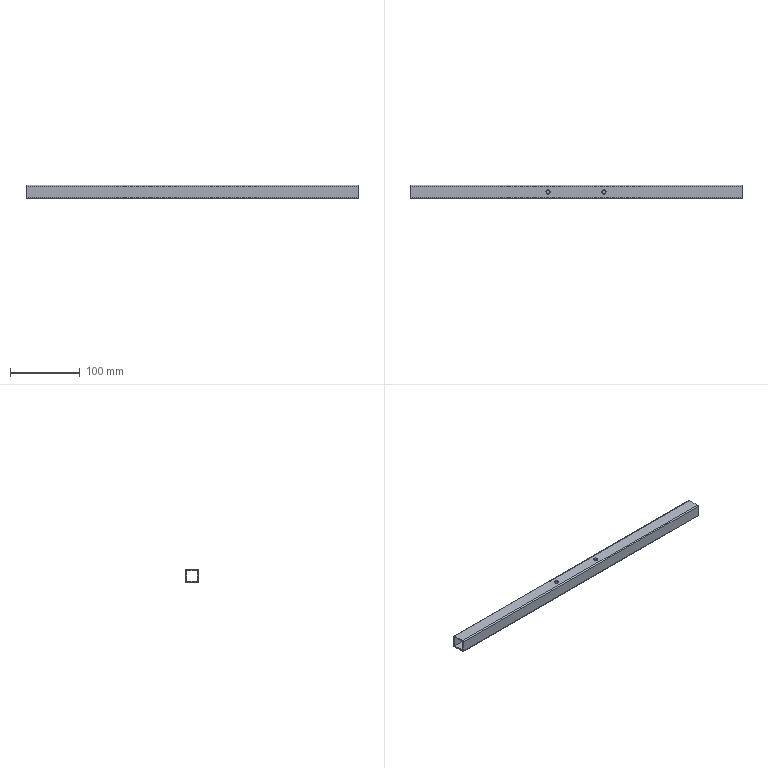Part | NX | features BREP 1 | 1 solid | 18 faces | box 474.98 x 19.05 x 19.05 mm | volume 63115 mm3 | plane 10 | cylinder 8 | commonest cylinder face diameters 3.175 x4 5.842 x4
STEP:
#1=CARTESIAN_POINT('',(-237.49,9.525,-7.938));
#2=VERTEX_POINT('',#1);
#3=CARTESIAN_POINT('',(-237.49,9.525,7.938));
#4=VERTEX_POINT('',#3);
#5=CARTESIAN_POINT('',(-237.49,9.525,-7.938));
#6=DIRECTION('',(0.,0.,1.));
#7=VECTOR('',#6,1000.);
#8=LINE('',#5,#7);
#9=EDGE_CURVE('',#2,#4,#8,.T.);
#10=ORIENTED_EDGE('',*,*,#9,.F.);
#11=CARTESIAN_POINT('',(-237.49,7.938,-9.525));
#12=VERTEX_POINT('',#11);
#13=CARTESIAN_POINT('',(-237.49,7.938,-7.938));
#14=DIRECTION('',(-1.,0.,0.));
#15=DIRECTION('',(0.,1.,0.));
#16=AXIS2_PLACEMENT_3D('',#13,#14,#15);
#17=CIRCLE('',#16,1.587);
#18=EDGE_CURVE('',#2,#12,#17,.T.);
#19=ORIENTED_EDGE('',*,*,#18,.T.);
#20=CARTESIAN_POINT('',(-237.49,-7.938,-9.525));
#21=VERTEX_POINT('',#20);
#22=CARTESIAN_POINT('',(-237.49,-7.938,-9.525));
#23=DIRECTION('',(0.,1.,0.));
#24=VECTOR('',#23,1000.);
#25=LINE('',#22,#24);
#26=EDGE_CURVE('',#21,#12,#25,.T.);
#27=ORIENTED_EDGE('',*,*,#26,.F.);
#28=CARTESIAN_POINT('',(-237.49,-9.525,-7.938));
#29=VERTEX_POINT('',#28);
#30=CARTESIAN_POINT('',(-237.49,-7.938,-7.938));
#31=DIRECTION('',(-1.,0.,0.));
#32=DIRECTION('',(0.,0.,-1.));
#33=AXIS2_PLACEMENT_3D('',#30,#31,#32);
#34=CIRCLE('',#33,1.587);
#35=EDGE_CURVE('',#21,#29,#34,.T.);
#36=ORIENTED_EDGE('',*,*,#35,.T.);
#37=CARTESIAN_POINT('',(-237.49,-9.525,7.938));
#38=VERTEX_POINT('',#37);
#39=CARTESIAN_POINT('',(-237.49,-9.525,7.938));
#40=DIRECTION('',(0.,0.,-1.));
#41=VECTOR('',#40,1000.);
#42=LINE('',#39,#41);
#43=EDGE_CURVE('',#38,#29,#42,.T.);
#44=ORIENTED_EDGE('',*,*,#43,.F.);
#45=CARTESIAN_POINT('',(-237.49,-7.938,9.525));
#46=VERTEX_POINT('',#45);
#47=CARTESIAN_POINT('',(-237.49,-7.938,7.938));
#48=DIRECTION('',(-1.,0.,0.));
#49=DIRECTION('',(0.,-1.,0.));
#50=AXIS2_PLACEMENT_3D('',#47,#48,#49);
#51=CIRCLE('',#50,1.587);
#52=EDGE_CURVE('',#38,#46,#51,.T.);
#53=ORIENTED_EDGE('',*,*,#52,.T.);
#54=CARTESIAN_POINT('',(-237.49,7.938,9.525));
#55=VERTEX_POINT('',#54);
#56=CARTESIAN_POINT('',(-237.49,7.938,9.525));
#57=DIRECTION('',(0.,-1.,0.));
#58=VECTOR('',#57,1000.);
#59=LINE('',#56,#58);
#60=EDGE_CURVE('',#55,#46,#59,.T.);
#61=ORIENTED_EDGE('',*,*,#60,.F.);
#62=CARTESIAN_POINT('',(-237.49,7.938,7.938));
#63=DIRECTION('',(-1.,0.,0.));
#64=DIRECTION('',(0.,0.,1.));
#65=AXIS2_PLACEMENT_3D('',#62,#63,#64);
#66=CIRCLE('',#65,1.587);
#67=EDGE_CURVE('',#55,#4,#66,.T.);
#68=ORIENTED_EDGE('',*,*,#67,.T.);
#69=EDGE_LOOP('',(#10,#19,#27,#36,#44,#53,#61,#68));
#70=FACE_BOUND('',#69,.T.);
#71=CARTESIAN_POINT('',(-237.49,7.544,7.544));
#72=VERTEX_POINT('',#71);
#73=CARTESIAN_POINT('',(-237.49,7.544,-7.544));
#74=VERTEX_POINT('',#73);
#75=CARTESIAN_POINT('',(-237.49,7.544,7.544));
#76=DIRECTION('',(0.,0.,-1.));
#77=VECTOR('',#76,1000.);
#78=LINE('',#75,#77);
#79=EDGE_CURVE('',#72,#74,#78,.T.);
#80=ORIENTED_EDGE('',*,*,#79,.F.);
#81=CARTESIAN_POINT('',(-237.49,-7.544,7.544));
#82=VERTEX_POINT('',#81);
#83=CARTESIAN_POINT('',(-237.49,-7.544,7.544));
#84=DIRECTION('',(0.,1.,0.));
#85=VECTOR('',#84,1000.);
#86=LINE('',#83,#85);
#87=EDGE_CURVE('',#82,#72,#86,.T.);
#88=ORIENTED_EDGE('',*,*,#87,.F.);
#89=CARTESIAN_POINT('',(-237.49,-7.544,-7.544));
#90=VERTEX_POINT('',#89);
#91=CARTESIAN_POINT('',(-237.49,-7.544,-7.544));
#92=DIRECTION('',(0.,0.,1.));
#93=VECTOR('',#92,1000.);
#94=LINE('',#91,#93);
#95=EDGE_CURVE('',#90,#82,#94,.T.);
#96=ORIENTED_EDGE('',*,*,#95,.F.);
#97=CARTESIAN_POINT('',(-237.49,7.544,-7.544));
#98=DIRECTION('',(0.,-1.,0.));
#99=VECTOR('',#98,1000.);
#100=LINE('',#97,#99);
#101=EDGE_CURVE('',#74,#90,#100,.T.);
#102=ORIENTED_EDGE('',*,*,#101,.F.);
#103=EDGE_LOOP('',(#80,#88,#96,#102));
#104=FACE_BOUND('',#103,.T.);
#105=CARTESIAN_POINT('',(-237.49,0.,0.));
#106=DIRECTION('',(1.,0.,0.));
#107=DIRECTION('',(0.,1.,0.));
#108=AXIS2_PLACEMENT_3D('',#105,#106,#107);
#109=PLANE('',#108);
#110=ADVANCED_FACE('',(#70,#104),#109,.F.);
#111=CARTESIAN_POINT('',(237.49,-7.544,-7.544));
#112=VERTEX_POINT('',#111);
#113=CARTESIAN_POINT('',(-237.49,-7.544,-7.544));
#114=DIRECTION('',(1.,0.,0.));
#115=VECTOR('',#114,1000.);
#116=LINE('',#113,#115);
#117=EDGE_CURVE('',#90,#112,#116,.T.);
#118=ORIENTED_EDGE('',*,*,#117,.T.);
#119=CARTESIAN_POINT('',(237.49,7.544,-7.544));
#120=VERTEX_POINT('',#119);
#121=CARTESIAN_POINT('',(237.49,7.544,-7.544));
#122=DIRECTION('',(0.,-1.,0.));
#123=VECTOR('',#122,1000.);
#124=LINE('',#121,#123);
#125=EDGE_CURVE('',#120,#112,#124,.T.);
#126=ORIENTED_EDGE('',*,*,#125,.F.);
#127=CARTESIAN_POINT('',(-237.49,7.544,-7.544));
#128=DIRECTION('',(1.,0.,0.));
#129=VECTOR('',#128,1000.);
#130=LINE('',#127,#129);
#131=EDGE_CURVE('',#74,#120,#130,.T.);
#132=ORIENTED_EDGE('',*,*,#131,.F.);
#133=ORIENTED_EDGE('',*,*,#101,.T.);
#134=EDGE_LOOP('',(#118,#126,#132,#133));
#135=FACE_BOUND('',#134,.T.);
#136=CARTESIAN_POINT('',(-237.49,7.544,-7.544));
#137=DIRECTION('',(0.,0.,1.));
#138=DIRECTION('',(1.,0.,0.));
#139=AXIS2_PLACEMENT_3D('',#136,#137,#138);
#140=PLANE('',#139);
#141=ADVANCED_FACE('',(#135),#140,.T.);
#142=ORIENTED_EDGE('',*,*,#131,.T.);
#143=CARTESIAN_POINT('',(237.49,7.544,7.544));
#144=VERTEX_POINT('',#143);
#145=CARTESIAN_POINT('',(237.49,7.544,7.544));
#146=DIRECTION('',(0.,0.,-1.));
#147=VECTOR('',#146,1000.);
#148=LINE('',#145,#147);
#149=EDGE_CURVE('',#144,#120,#148,.T.);
#150=ORIENTED_EDGE('',*,*,#149,.F.);
#151=CARTESIAN_POINT('',(-237.49,7.544,7.544));
#152=DIRECTION('',(1.,0.,0.));
#153=VECTOR('',#152,1000.);
#154=LINE('',#151,#153);
#155=EDGE_CURVE('',#72,#144,#154,.T.);
#156=ORIENTED_EDGE('',*,*,#155,.F.);
#157=ORIENTED_EDGE('',*,*,#79,.T.);
#158=EDGE_LOOP('',(#142,#150,#156,#157));
#159=FACE_BOUND('',#158,.T.);
#160=CARTESIAN_POINT('',(-237.49,7.544,7.544));
#161=DIRECTION('',(0.,-1.,0.));
#162=DIRECTION('',(0.,0.,-1.));
#163=AXIS2_PLACEMENT_3D('',#160,#161,#162);
#164=PLANE('',#163);
#165=ADVANCED_FACE('',(#159),#164,.T.);
#166=ORIENTED_EDGE('',*,*,#155,.T.);
#167=CARTESIAN_POINT('',(237.49,-7.544,7.544));
#168=VERTEX_POINT('',#167);
#169=CARTESIAN_POINT('',(237.49,-7.544,7.544));
#170=DIRECTION('',(0.,1.,0.));
#171=VECTOR('',#170,1000.);
#172=LINE('',#169,#171);
#173=EDGE_CURVE('',#168,#144,#172,.T.);
#174=ORIENTED_EDGE('',*,*,#173,.F.);
#175=CARTESIAN_POINT('',(-237.49,-7.544,7.544));
#176=DIRECTION('',(1.,0.,0.));
#177=VECTOR('',#176,1000.);
#178=LINE('',#175,#177);
#179=EDGE_CURVE('',#82,#168,#178,.T.);
#180=ORIENTED_EDGE('',*,*,#179,.F.);
#181=ORIENTED_EDGE('',*,*,#87,.T.);
#182=EDGE_LOOP('',(#166,#174,#180,#181));
#183=FACE_BOUND('',#182,.T.);
#184=CARTESIAN_POINT('',(-37.084,0.,7.544));
#185=VERTEX_POINT('',#184);
#186=CARTESIAN_POINT('',(-42.926,0.,7.544));
#187=VERTEX_POINT('',#186);
#188=CARTESIAN_POINT('',(-40.005,0.,7.544));
#189=DIRECTION('',(0.,0.,-1.));
#190=DIRECTION('',(1.,0.,0.));
#191=AXIS2_PLACEMENT_3D('',#188,#189,#190);
#192=CIRCLE('',#191,2.921);
#193=EDGE_CURVE('',#185,#187,#192,.T.);
#194=ORIENTED_EDGE('',*,*,#193,.F.);
#195=CARTESIAN_POINT('',(-40.005,0.,7.544));
#196=DIRECTION('',(0.,0.,-1.));
#197=DIRECTION('',(-1.,0.,0.));
#198=AXIS2_PLACEMENT_3D('',#195,#196,#197);
#199=CIRCLE('',#198,2.921);
#200=EDGE_CURVE('',#187,#185,#199,.T.);
#201=ORIENTED_EDGE('',*,*,#200,.F.);
#202=EDGE_LOOP('',(#194,#201));
#203=FACE_BOUND('',#202,.T.);
#204=CARTESIAN_POINT('',(42.926,0.,7.544));
#205=VERTEX_POINT('',#204);
#206=CARTESIAN_POINT('',(37.084,0.,7.544));
#207=VERTEX_POINT('',#206);
#208=CARTESIAN_POINT('',(40.005,0.,7.544));
#209=DIRECTION('',(0.,0.,-1.));
#210=DIRECTION('',(1.,0.,0.));
#211=AXIS2_PLACEMENT_3D('',#208,#209,#210);
#212=CIRCLE('',#211,2.921);
#213=EDGE_CURVE('',#205,#207,#212,.T.);
#214=ORIENTED_EDGE('',*,*,#213,.F.);
#215=CARTESIAN_POINT('',(40.005,0.,7.544));
#216=DIRECTION('',(0.,0.,-1.));
#217=DIRECTION('',(-1.,0.,0.));
#218=AXIS2_PLACEMENT_3D('',#215,#216,#217);
#219=CIRCLE('',#218,2.921);
#220=EDGE_CURVE('',#207,#205,#219,.T.);
#221=ORIENTED_EDGE('',*,*,#220,.F.);
#222=EDGE_LOOP('',(#214,#221));
#223=FACE_BOUND('',#222,.T.);
#224=CARTESIAN_POINT('',(-237.49,-7.544,7.544));
#225=DIRECTION('',(0.,0.,-1.));
#226=DIRECTION('',(0.,-1.,0.));
#227=AXIS2_PLACEMENT_3D('',#224,#225,#226);
#228=PLANE('',#227);
#229=ADVANCED_FACE('',(#183,#203,#223),#228,.T.);
#230=ORIENTED_EDGE('',*,*,#179,.T.);
#231=CARTESIAN_POINT('',(237.49,-7.544,-7.544));
#232=DIRECTION('',(0.,0.,1.));
#233=VECTOR('',#232,1000.);
#234=LINE('',#231,#233);
#235=EDGE_CURVE('',#112,#168,#234,.T.);
#236=ORIENTED_EDGE('',*,*,#235,.F.);
#237=ORIENTED_EDGE('',*,*,#117,.F.);
#238=ORIENTED_EDGE('',*,*,#95,.T.);
#239=EDGE_LOOP('',(#230,#236,#237,#238));
#240=FACE_BOUND('',#239,.T.);
#241=CARTESIAN_POINT('',(-237.49,-7.544,-7.544));
#242=DIRECTION('',(0.,1.,0.));
#243=DIRECTION('',(1.,0.,0.));
#244=AXIS2_PLACEMENT_3D('',#241,#242,#243);
#245=PLANE('',#244);
#246=ADVANCED_FACE('',(#240),#245,.T.);
#247=CARTESIAN_POINT('',(237.49,7.938,9.525));
#248=VERTEX_POINT('',#247);
#249=CARTESIAN_POINT('',(237.49,-7.938,9.525));
#250=VERTEX_POINT('',#249);
#251=CARTESIAN_POINT('',(237.49,7.938,9.525));
#252=DIRECTION('',(0.,-1.,0.));
#253=VECTOR('',#252,1000.);
#254=LINE('',#251,#253);
#255=EDGE_CURVE('',#248,#250,#254,.T.);
#256=ORIENTED_EDGE('',*,*,#255,.T.);
#257=CARTESIAN_POINT('',(237.49,-9.525,7.938));
#258=VERTEX_POINT('',#257);
#259=CARTESIAN_POINT('',(237.49,-7.938,7.938));
#260=DIRECTION('',(1.,0.,0.));
#261=DIRECTION('',(0.,0.,1.));
#262=AXIS2_PLACEMENT_3D('',#259,#260,#261);
#263=CIRCLE('',#262,1.587);
#264=EDGE_CURVE('',#250,#258,#263,.T.);
#265=ORIENTED_EDGE('',*,*,#264,.T.);
#266=CARTESIAN_POINT('',(237.49,-9.525,-7.938));
#267=VERTEX_POINT('',#266);
#268=CARTESIAN_POINT('',(237.49,-9.525,7.938));
#269=DIRECTION('',(0.,0.,-1.));
#270=VECTOR('',#269,1000.);
#271=LINE('',#268,#270);
#272=EDGE_CURVE('',#258,#267,#271,.T.);
#273=ORIENTED_EDGE('',*,*,#272,.T.);
#274=CARTESIAN_POINT('',(237.49,-7.938,-9.525));
#275=VERTEX_POINT('',#274);
#276=CARTESIAN_POINT('',(237.49,-7.938,-7.938));
#277=DIRECTION('',(1.,0.,0.));
#278=DIRECTION('',(0.,-1.,0.));
#279=AXIS2_PLACEMENT_3D('',#276,#277,#278);
#280=CIRCLE('',#279,1.587);
#281=EDGE_CURVE('',#267,#275,#280,.T.);
#282=ORIENTED_EDGE('',*,*,#281,.T.);
#283=CARTESIAN_POINT('',(237.49,7.938,-9.525));
#284=VERTEX_POINT('',#283);
#285=CARTESIAN_POINT('',(237.49,-7.938,-9.525));
#286=DIRECTION('',(0.,1.,0.));
#287=VECTOR('',#286,1000.);
#288=LINE('',#285,#287);
#289=EDGE_CURVE('',#275,#284,#288,.T.);
#290=ORIENTED_EDGE('',*,*,#289,.T.);
#291=CARTESIAN_POINT('',(237.49,9.525,-7.938));
#292=VERTEX_POINT('',#291);
#293=CARTESIAN_POINT('',(237.49,7.938,-7.938));
#294=DIRECTION('',(1.,0.,0.));
#295=DIRECTION('',(0.,0.,-1.));
#296=AXIS2_PLACEMENT_3D('',#293,#294,#295);
#297=CIRCLE('',#296,1.587);
#298=EDGE_CURVE('',#284,#292,#297,.T.);
#299=ORIENTED_EDGE('',*,*,#298,.T.);
#300=CARTESIAN_POINT('',(237.49,9.525,7.938));
#301=VERTEX_POINT('',#300);
#302=CARTESIAN_POINT('',(237.49,9.525,-7.938));
#303=DIRECTION('',(0.,0.,1.));
#304=VECTOR('',#303,1000.);
#305=LINE('',#302,#304);
#306=EDGE_CURVE('',#292,#301,#305,.T.);
#307=ORIENTED_EDGE('',*,*,#306,.T.);
#308=CARTESIAN_POINT('',(237.49,7.938,7.938));
#309=DIRECTION('',(1.,0.,0.));
#310=DIRECTION('',(0.,1.,0.));
#311=AXIS2_PLACEMENT_3D('',#308,#309,#310);
#312=CIRCLE('',#311,1.587);
#313=EDGE_CURVE('',#301,#248,#312,.T.);
#314=ORIENTED_EDGE('',*,*,#313,.T.);
#315=EDGE_LOOP('',(#256,#265,#273,#282,#290,#299,#307,#314));
#316=FACE_BOUND('',#315,.T.);
#317=ORIENTED_EDGE('',*,*,#235,.T.);
#318=ORIENTED_EDGE('',*,*,#173,.T.);
#319=ORIENTED_EDGE('',*,*,#149,.T.);
#320=ORIENTED_EDGE('',*,*,#125,.T.);
#321=EDGE_LOOP('',(#317,#318,#319,#320));
#322=FACE_BOUND('',#321,.T.);
#323=CARTESIAN_POINT('',(237.49,0.,0.));
#324=DIRECTION('',(1.,0.,0.));
#325=DIRECTION('',(0.,1.,0.));
#326=AXIS2_PLACEMENT_3D('',#323,#324,#325);
#327=PLANE('',#326);
#328=ADVANCED_FACE('',(#316,#322),#327,.T.);
#329=ORIENTED_EDGE('',*,*,#313,.F.);
#330=CARTESIAN_POINT('',(237.49,9.525,7.938));
#331=DIRECTION('',(-1.,0.,0.));
#332=VECTOR('',#331,1000.);
#333=LINE('',#330,#332);
#334=EDGE_CURVE('',#301,#4,#333,.T.);
#335=ORIENTED_EDGE('',*,*,#334,.T.);
#336=ORIENTED_EDGE('',*,*,#67,.F.);
#337=CARTESIAN_POINT('',(237.49,7.938,9.525));
#338=DIRECTION('',(-1.,0.,0.));
#339=VECTOR('',#338,1000.);
#340=LINE('',#337,#339);
#341=EDGE_CURVE('',#248,#55,#340,.T.);
#342=ORIENTED_EDGE('',*,*,#341,.F.);
#343=EDGE_LOOP('',(#329,#335,#336,#342));
#344=FACE_BOUND('',#343,.T.);
#345=CARTESIAN_POINT('',(238.234,7.938,7.938));
#346=DIRECTION('',(-1.,0.,0.));
#347=DIRECTION('',(0.,0.,1.));
#348=AXIS2_PLACEMENT_3D('',#345,#346,#347);
#349=CYLINDRICAL_SURFACE('',#348,1.587);
#350=ADVANCED_FACE('',(#344),#349,.T.);
#351=ORIENTED_EDGE('',*,*,#60,.T.);
#352=CARTESIAN_POINT('',(237.49,-7.938,9.525));
#353=DIRECTION('',(-1.,0.,0.));
#354=VECTOR('',#353,1000.);
#355=LINE('',#352,#354);
#356=EDGE_CURVE('',#250,#46,#355,.T.);
#357=ORIENTED_EDGE('',*,*,#356,.F.);
#358=ORIENTED_EDGE('',*,*,#255,.F.);
#359=ORIENTED_EDGE('',*,*,#341,.T.);
#360=EDGE_LOOP('',(#351,#357,#358,#359));
#361=FACE_BOUND('',#360,.T.);
#362=CARTESIAN_POINT('',(-37.084,0.,9.525));
#363=VERTEX_POINT('',#362);
#364=CARTESIAN_POINT('',(-42.926,0.,9.525));
#365=VERTEX_POINT('',#364);
#366=CARTESIAN_POINT('',(-40.005,0.,9.525));
#367=DIRECTION('',(0.,0.,-1.));
#368=DIRECTION('',(1.,0.,0.));
#369=AXIS2_PLACEMENT_3D('',#366,#367,#368);
#370=CIRCLE('',#369,2.921);
#371=EDGE_CURVE('',#363,#365,#370,.T.);
#372=ORIENTED_EDGE('',*,*,#371,.T.);
#373=CARTESIAN_POINT('',(-40.005,0.,9.525));
#374=DIRECTION('',(0.,0.,-1.));
#375=DIRECTION('',(-1.,0.,0.));
#376=AXIS2_PLACEMENT_3D('',#373,#374,#375);
#377=CIRCLE('',#376,2.921);
#378=EDGE_CURVE('',#365,#363,#377,.T.);
#379=ORIENTED_EDGE('',*,*,#378,.T.);
#380=EDGE_LOOP('',(#372,#379));
#381=FACE_BOUND('',#380,.T.);
#382=CARTESIAN_POINT('',(42.926,0.,9.525));
#383=VERTEX_POINT('',#382);
#384=CARTESIAN_POINT('',(37.084,0.,9.525));
#385=VERTEX_POINT('',#384);
#386=CARTESIAN_POINT('',(40.005,0.,9.525));
#387=DIRECTION('',(0.,0.,-1.));
#388=DIRECTION('',(1.,0.,0.));
#389=AXIS2_PLACEMENT_3D('',#386,#387,#388);
#390=CIRCLE('',#389,2.921);
#391=EDGE_CURVE('',#383,#385,#390,.T.);
#392=ORIENTED_EDGE('',*,*,#391,.T.);
#393=CARTESIAN_POINT('',(40.005,0.,9.525));
#394=DIRECTION('',(0.,0.,-1.));
#395=DIRECTION('',(-1.,0.,0.));
#396=AXIS2_PLACEMENT_3D('',#393,#394,#395);
#397=CIRCLE('',#396,2.921);
#398=EDGE_CURVE('',#385,#383,#397,.T.);
#399=ORIENTED_EDGE('',*,*,#398,.T.);
#400=EDGE_LOOP('',(#392,#399));
#401=FACE_BOUND('',#400,.T.);
#402=CARTESIAN_POINT('',(-237.49,9.525,9.525));
#403=DIRECTION('',(0.,0.,1.));
#404=DIRECTION('',(1.,0.,0.));
#405=AXIS2_PLACEMENT_3D('',#402,#403,#404);
#406=PLANE('',#405);
#407=ADVANCED_FACE('',(#361,#381,#401),#406,.T.);
#408=ORIENTED_EDGE('',*,*,#264,.F.);
#409=ORIENTED_EDGE('',*,*,#356,.T.);
#410=ORIENTED_EDGE('',*,*,#52,.F.);
#411=CARTESIAN_POINT('',(237.49,-9.525,7.938));
#412=DIRECTION('',(-1.,0.,0.));
#413=VECTOR('',#412,1000.);
#414=LINE('',#411,#413);
#415=EDGE_CURVE('',#258,#38,#414,.T.);
#416=ORIENTED_EDGE('',*,*,#415,.F.);
#417=EDGE_LOOP('',(#408,#409,#410,#416));
#418=FACE_BOUND('',#417,.T.);
#419=CARTESIAN_POINT('',(238.234,-7.938,7.938));
#420=DIRECTION('',(-1.,0.,0.));
#421=DIRECTION('',(0.,-1.,0.));
#422=AXIS2_PLACEMENT_3D('',#419,#420,#421);
#423=CYLINDRICAL_SURFACE('',#422,1.587);
#424=ADVANCED_FACE('',(#418),#423,.T.);
#425=ORIENTED_EDGE('',*,*,#43,.T.);
#426=CARTESIAN_POINT('',(237.49,-9.525,-7.938));
#427=DIRECTION('',(-1.,0.,0.));
#428=VECTOR('',#427,1000.);
#429=LINE('',#426,#428);
#430=EDGE_CURVE('',#267,#29,#429,.T.);
#431=ORIENTED_EDGE('',*,*,#430,.F.);
#432=ORIENTED_EDGE('',*,*,#272,.F.);
#433=ORIENTED_EDGE('',*,*,#415,.T.);
#434=EDGE_LOOP('',(#425,#431,#432,#433));
#435=FACE_BOUND('',#434,.T.);
#436=CARTESIAN_POINT('',(-237.49,-9.525,9.525));
#437=DIRECTION('',(0.,-1.,0.));
#438=DIRECTION('',(0.,0.,-1.));
#439=AXIS2_PLACEMENT_3D('',#436,#437,#438);
#440=PLANE('',#439);
#441=ADVANCED_FACE('',(#435),#440,.T.);
#442=ORIENTED_EDGE('',*,*,#281,.F.);
#443=ORIENTED_EDGE('',*,*,#430,.T.);
#444=ORIENTED_EDGE('',*,*,#35,.F.);
#445=CARTESIAN_POINT('',(237.49,-7.938,-9.525));
#446=DIRECTION('',(-1.,0.,0.));
#447=VECTOR('',#446,1000.);
#448=LINE('',#445,#447);
#449=EDGE_CURVE('',#275,#21,#448,.T.);
#450=ORIENTED_EDGE('',*,*,#449,.F.);
#451=EDGE_LOOP('',(#442,#443,#444,#450));
#452=FACE_BOUND('',#451,.T.);
#453=CARTESIAN_POINT('',(238.234,-7.938,-7.938));
#454=DIRECTION('',(-1.,0.,0.));
#455=DIRECTION('',(0.,0.,-1.));
#456=AXIS2_PLACEMENT_3D('',#453,#454,#455);
#457=CYLINDRICAL_SURFACE('',#456,1.587);
#458=ADVANCED_FACE('',(#452),#457,.T.);
#459=ORIENTED_EDGE('',*,*,#289,.F.);
#460=ORIENTED_EDGE('',*,*,#449,.T.);
#461=ORIENTED_EDGE('',*,*,#26,.T.);
#462=CARTESIAN_POINT('',(237.49,7.938,-9.525));
#463=DIRECTION('',(-1.,0.,0.));
#464=VECTOR('',#463,1000.);
#465=LINE('',#462,#464);
#466=EDGE_CURVE('',#284,#12,#465,.T.);
#467=ORIENTED_EDGE('',*,*,#466,.F.);
#468=EDGE_LOOP('',(#459,#460,#461,#467));
#469=FACE_BOUND('',#468,.T.);
#470=CARTESIAN_POINT('',(-237.49,-9.525,-9.525));
#471=DIRECTION('',(0.,0.,-1.));
#472=DIRECTION('',(0.,-1.,0.));
#473=AXIS2_PLACEMENT_3D('',#470,#471,#472);
#474=PLANE('',#473);
#475=ADVANCED_FACE('',(#469),#474,.T.);
#476=ORIENTED_EDGE('',*,*,#298,.F.);
#477=ORIENTED_EDGE('',*,*,#466,.T.);
#478=ORIENTED_EDGE('',*,*,#18,.F.);
#479=CARTESIAN_POINT('',(237.49,9.525,-7.938));
#480=DIRECTION('',(-1.,0.,0.));
#481=VECTOR('',#480,1000.);
#482=LINE('',#479,#481);
#483=EDGE_CURVE('',#292,#2,#482,.T.);
#484=ORIENTED_EDGE('',*,*,#483,.F.);
#485=EDGE_LOOP('',(#476,#477,#478,#484));
#486=FACE_BOUND('',#485,.T.);
#487=CARTESIAN_POINT('',(238.234,7.938,-7.938));
#488=DIRECTION('',(-1.,0.,0.));
#489=DIRECTION('',(0.,1.,0.));
#490=AXIS2_PLACEMENT_3D('',#487,#488,#489);
#491=CYLINDRICAL_SURFACE('',#490,1.587);
#492=ADVANCED_FACE('',(#486),#491,.T.);
#493=ORIENTED_EDGE('',*,*,#306,.F.);
#494=ORIENTED_EDGE('',*,*,#483,.T.);
#495=ORIENTED_EDGE('',*,*,#9,.T.);
#496=ORIENTED_EDGE('',*,*,#334,.F.);
#497=EDGE_LOOP('',(#493,#494,#495,#496));
#498=FACE_BOUND('',#497,.T.);
#499=CARTESIAN_POINT('',(-237.49,9.525,-9.525));
#500=DIRECTION('',(0.,1.,0.));
#501=DIRECTION('',(1.,0.,0.));
#502=AXIS2_PLACEMENT_3D('',#499,#500,#501);
#503=PLANE('',#502);
#504=ADVANCED_FACE('',(#498),#503,.T.);
#505=CARTESIAN_POINT('',(-42.926,0.,9.525));
#506=DIRECTION('',(0.,0.,-1.));
#507=VECTOR('',#506,1000.);
#508=LINE('',#505,#507);
#509=EDGE_CURVE('',#365,#187,#508,.T.);
#510=ORIENTED_EDGE('',*,*,#509,.T.);
#511=ORIENTED_EDGE('',*,*,#200,.T.);
#512=CARTESIAN_POINT('',(-37.084,0.,9.525));
#513=DIRECTION('',(0.,0.,-1.));
#514=VECTOR('',#513,1000.);
#515=LINE('',#512,#514);
#516=EDGE_CURVE('',#363,#185,#515,.T.);
#517=ORIENTED_EDGE('',*,*,#516,.F.);
#518=ORIENTED_EDGE('',*,*,#378,.F.);
#519=EDGE_LOOP('',(#510,#511,#517,#518));
#520=FACE_BOUND('',#519,.T.);
#521=CARTESIAN_POINT('',(-40.005,0.,9.525));
#522=DIRECTION('',(0.,0.,-1.));
#523=DIRECTION('',(-1.,0.,0.));
#524=AXIS2_PLACEMENT_3D('',#521,#522,#523);
#525=CYLINDRICAL_SURFACE('',#524,2.921);
#526=ADVANCED_FACE('',(#520),#525,.F.);
#527=ORIENTED_EDGE('',*,*,#516,.T.);
#528=ORIENTED_EDGE('',*,*,#193,.T.);
#529=ORIENTED_EDGE('',*,*,#509,.F.);
#530=ORIENTED_EDGE('',*,*,#371,.F.);
#531=EDGE_LOOP('',(#527,#528,#529,#530));
#532=FACE_BOUND('',#531,.T.);
#533=CARTESIAN_POINT('',(-40.005,0.,9.525));
#534=DIRECTION('',(0.,0.,-1.));
#535=DIRECTION('',(-1.,0.,0.));
#536=AXIS2_PLACEMENT_3D('',#533,#534,#535);
#537=CYLINDRICAL_SURFACE('',#536,2.921);
#538=ADVANCED_FACE('',(#532),#537,.F.);
#539=CARTESIAN_POINT('',(37.084,0.,9.525));
#540=DIRECTION('',(0.,0.,-1.));
#541=VECTOR('',#540,1000.);
#542=LINE('',#539,#541);
#543=EDGE_CURVE('',#385,#207,#542,.T.);
#544=ORIENTED_EDGE('',*,*,#543,.T.);
#545=ORIENTED_EDGE('',*,*,#220,.T.);
#546=CARTESIAN_POINT('',(42.926,0.,9.525));
#547=DIRECTION('',(0.,0.,-1.));
#548=VECTOR('',#547,1000.);
#549=LINE('',#546,#548);
#550=EDGE_CURVE('',#383,#205,#549,.T.);
#551=ORIENTED_EDGE('',*,*,#550,.F.);
#552=ORIENTED_EDGE('',*,*,#398,.F.);
#553=EDGE_LOOP('',(#544,#545,#551,#552));
#554=FACE_BOUND('',#553,.T.);
#555=CARTESIAN_POINT('',(40.005,0.,9.525));
#556=DIRECTION('',(0.,0.,-1.));
#557=DIRECTION('',(-1.,0.,0.));
#558=AXIS2_PLACEMENT_3D('',#555,#556,#557);
#559=CYLINDRICAL_SURFACE('',#558,2.921);
#560=ADVANCED_FACE('',(#554),#559,.F.);
#561=ORIENTED_EDGE('',*,*,#550,.T.);
#562=ORIENTED_EDGE('',*,*,#213,.T.);
#563=ORIENTED_EDGE('',*,*,#543,.F.);
#564=ORIENTED_EDGE('',*,*,#391,.F.);
#565=EDGE_LOOP('',(#561,#562,#563,#564));
#566=FACE_BOUND('',#565,.T.);
#567=CARTESIAN_POINT('',(40.005,0.,9.525));
#568=DIRECTION('',(0.,0.,-1.));
#569=DIRECTION('',(-1.,0.,0.));
#570=AXIS2_PLACEMENT_3D('',#567,#568,#569);
#571=CYLINDRICAL_SURFACE('',#570,2.921);
#572=ADVANCED_FACE('',(#566),#571,.F.);
#573=CLOSED_SHELL('',(#110,#141,#165,#229,#246,#328,#350,#407,#424,#441,#458,#475,#492,#504,#526,#538,#560,#572));
#574=MANIFOLD_SOLID_BREP('',#573);
#575=(LENGTH_UNIT()NAMED_UNIT(*)SI_UNIT(.MILLI.,.METRE.));
#576=UNCERTAINTY_MEASURE_WITH_UNIT(LENGTH_MEASURE(0.00001),#575,'','');
#577=(NAMED_UNIT(*)PLANE_ANGLE_UNIT()SI_UNIT($,.RADIAN.));
#578=(NAMED_UNIT(*)SI_UNIT($,.STERADIAN.)SOLID_ANGLE_UNIT());
#579=(GEOMETRIC_REPRESENTATION_CONTEXT(3)GLOBAL_UNCERTAINTY_ASSIGNED_CONTEXT((#576))GLOBAL_UNIT_ASSIGNED_CONTEXT((#575,#577,#578))REPRESENTATION_CONTEXT('',''));
#580=ADVANCED_BREP_SHAPE_REPRESENTATION('',(#574),#579);